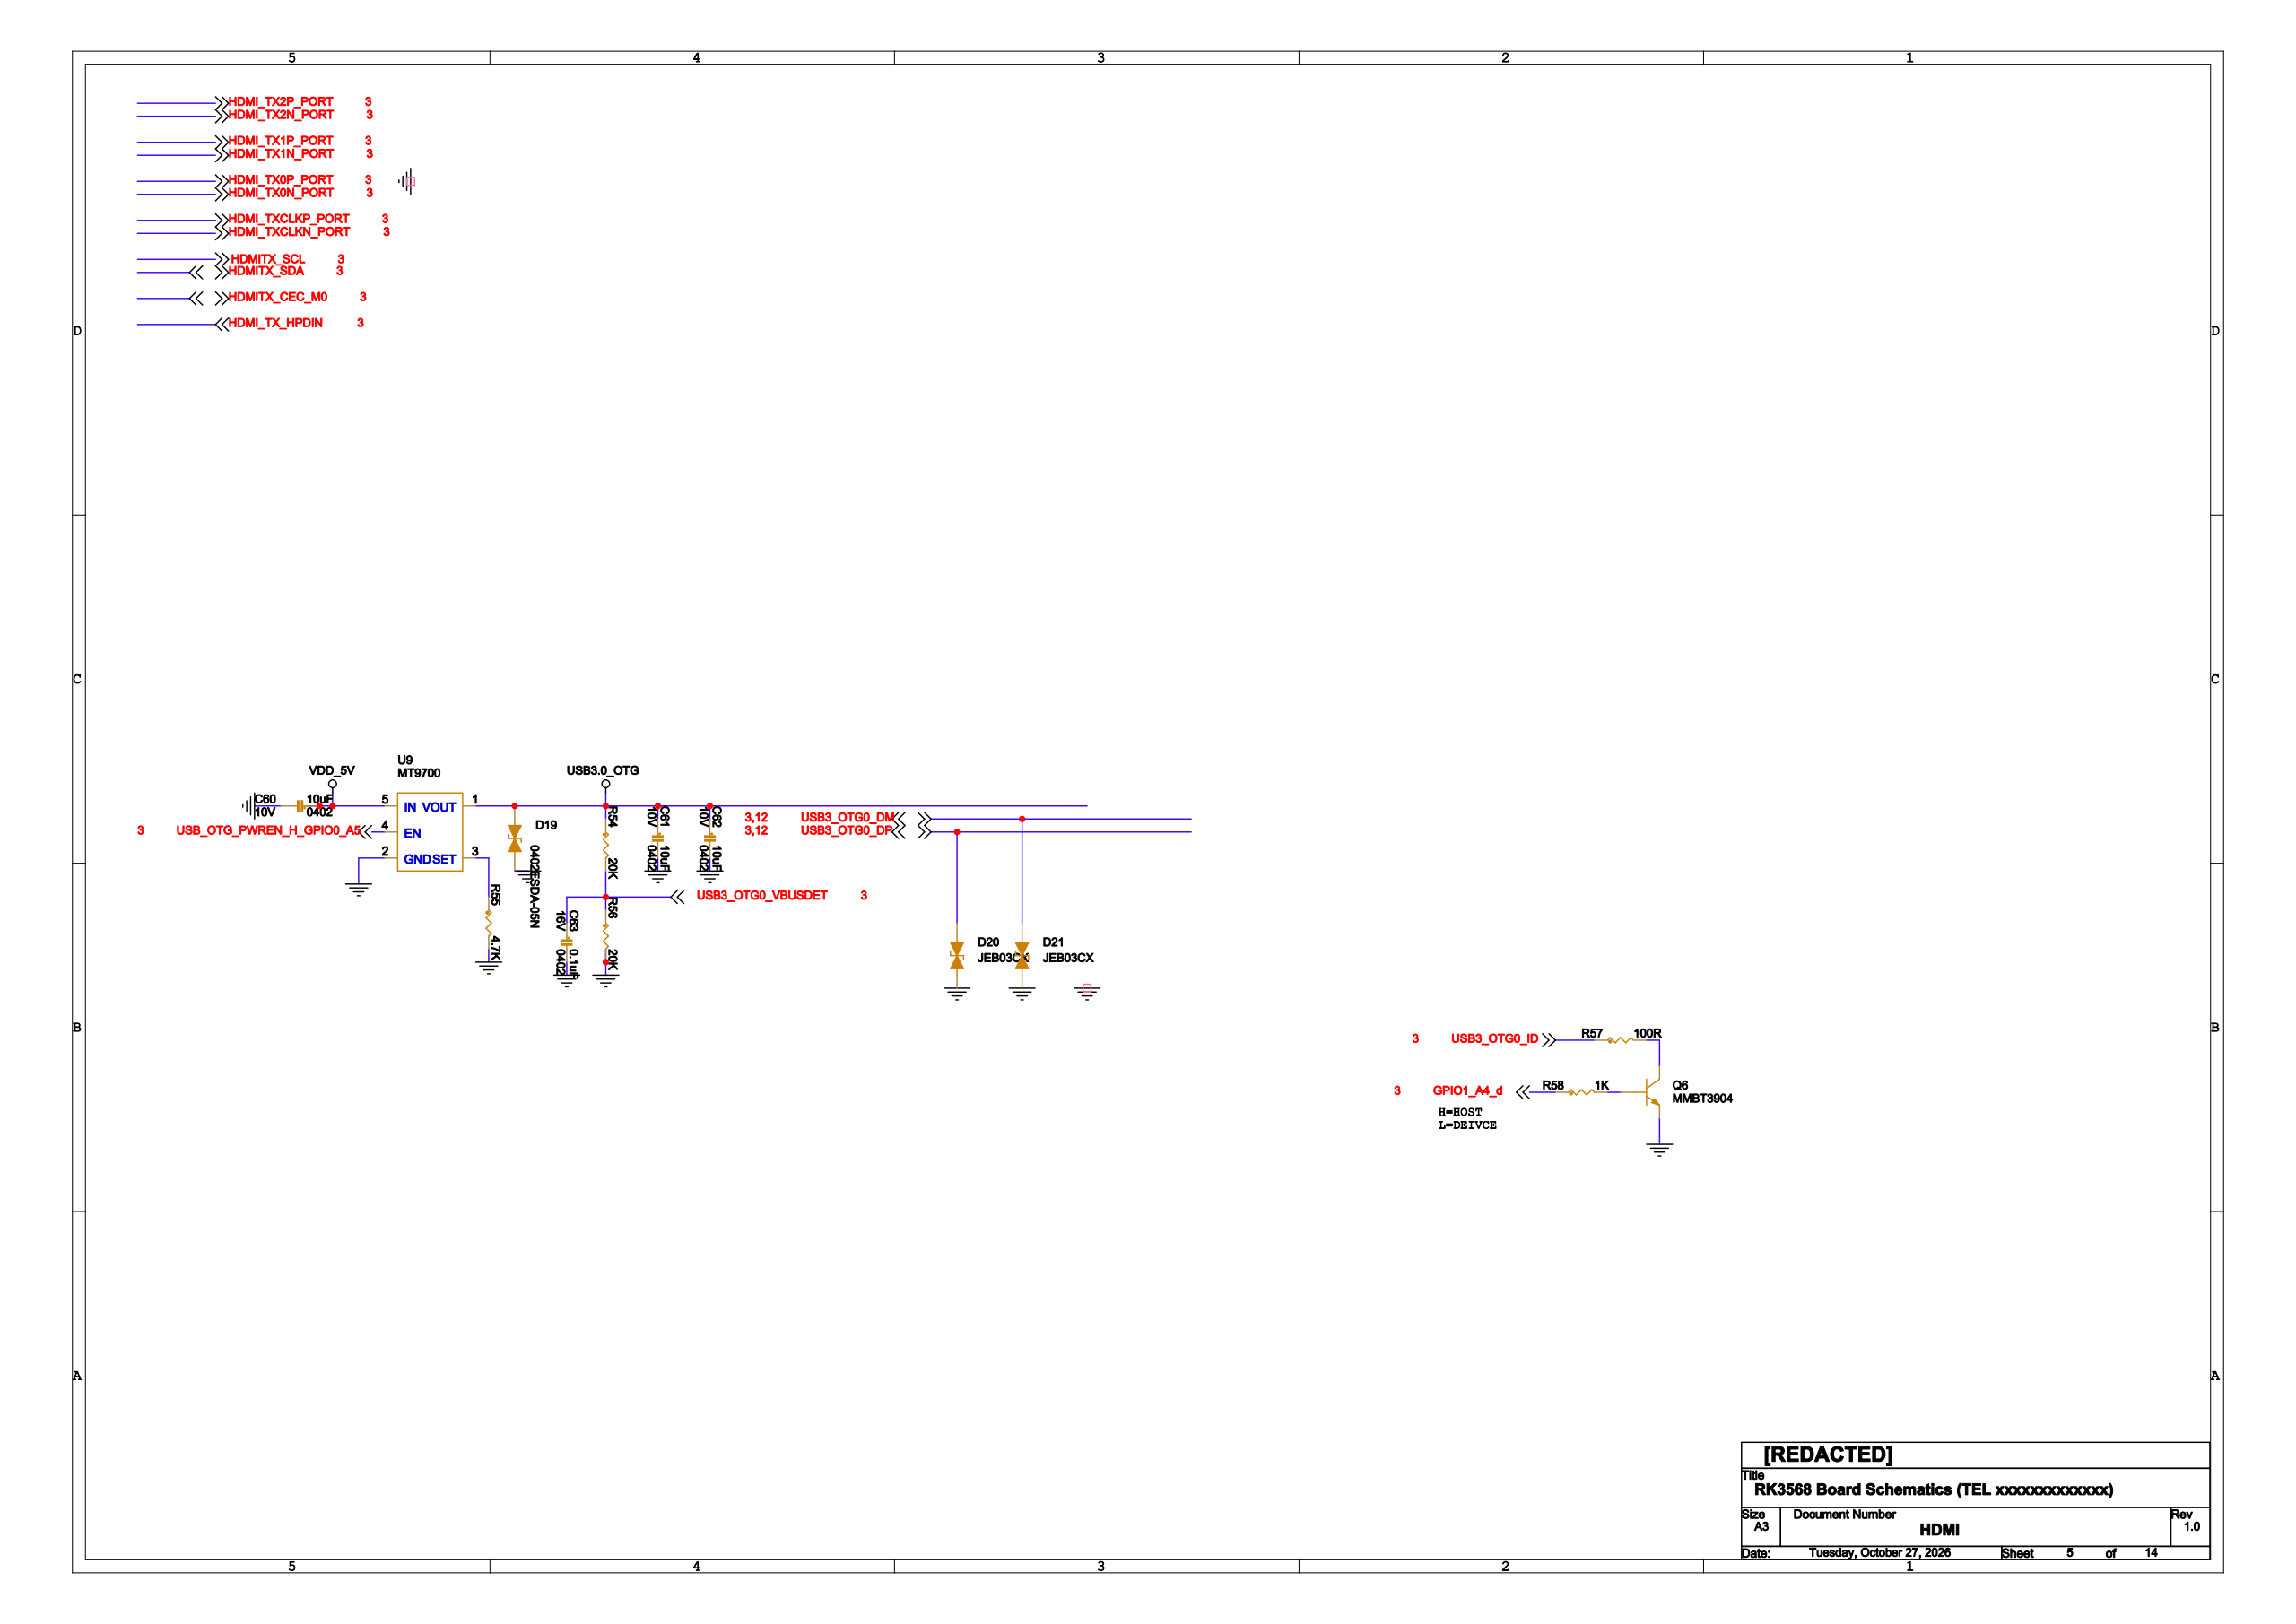Circuit board | Cadence Allegro | 669 parts | 581 nets | one sheet of the schematic
Parts on this sheet (reference | value | footprint):
C60 | 10uF | C0402
C61 | 10uF | C0402
C62 | 10uF | C0402
C63 | 0.1uF | C0402
D19 | 0402ESDA-05N | R0402
D20 | JEB03CX | SOD323
D21 | JEB03CX | SOD323
Q6 | MMBT3904 | SOT-23
R54 | 20K | R0402
R55 | 4.7K | R0402
R56 | 20K | R0402
R57 | 100R | R0402
R58 | 1K | R0402
U9 | MT9700 | SOT23-5
Nets of these parts (net: part-pin ...):
GND: C60-2 C61-2 C62-2 C63-2 D19-2 D20-1 D21-1 Q6-2 R55-2 R56-2 U9-2
VDD_5V: C60-1 U9-5
USB3_OTG0_VBUSDET: C63-1 R54-2 R56-1
USB3.0_OTG: C61-1 C62-1 D19-1 R54-1 U9-1
USB3_OTG0_DP: D20-2
USB3_OTG0_DM: D21-2
USB3_OTG0_ID: R57-1
N84557983: Q6-3 R57-2
GPIO1_A4_D: R58-1
N84002725: Q6-1 R58-2
N83865783: R55-1 U9-3
USB_OTG_PWREN_H_GPIO0_A5: U9-4